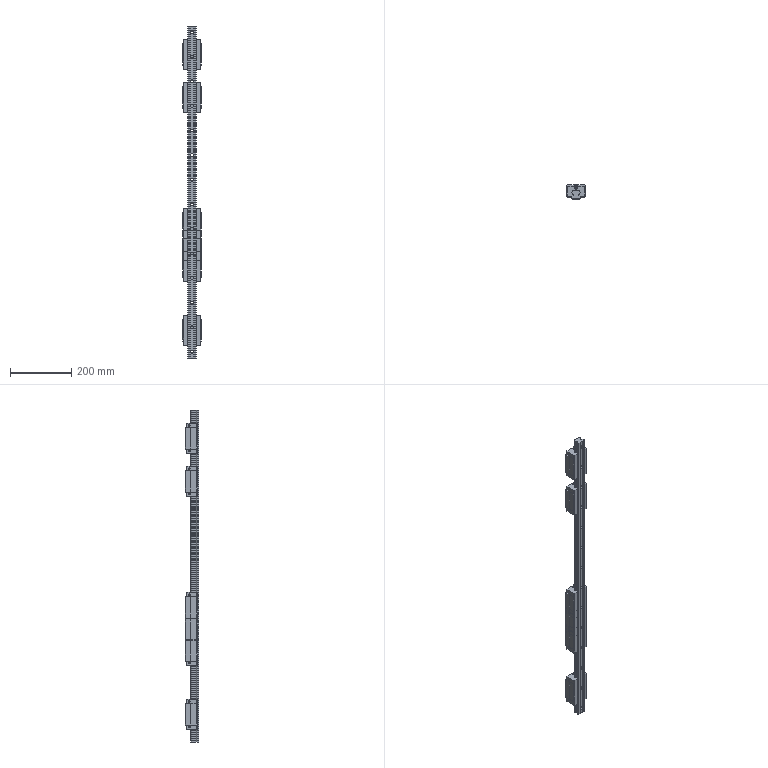Part | SolidWorks | 7 solids | 962 faces | box 60 x 45 x 1080 mm | volume 1638372 mm3 | plane 560 | cylinder 402 | commonest cylinder face diameters 1.2 x84 1 x48 5 x48 8 x48 1.6 x30 5.66 x28